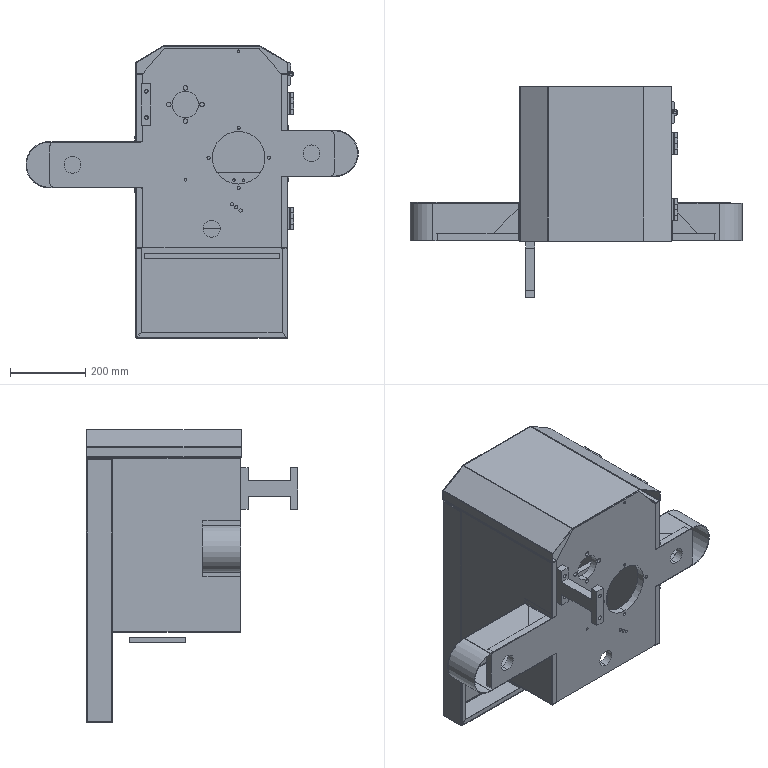Part | SolidWorks | 34 solids | 731 faces | box 883 x 562 x 778 mm | volume 14774515 mm3 | plane 359 | cylinder 324 | cone 32 | spline 16 | commonest cylinder face diameters 6.8 x44 8.5 x42 7.5 x40 15 x40 8.4 x32 1.473 x22